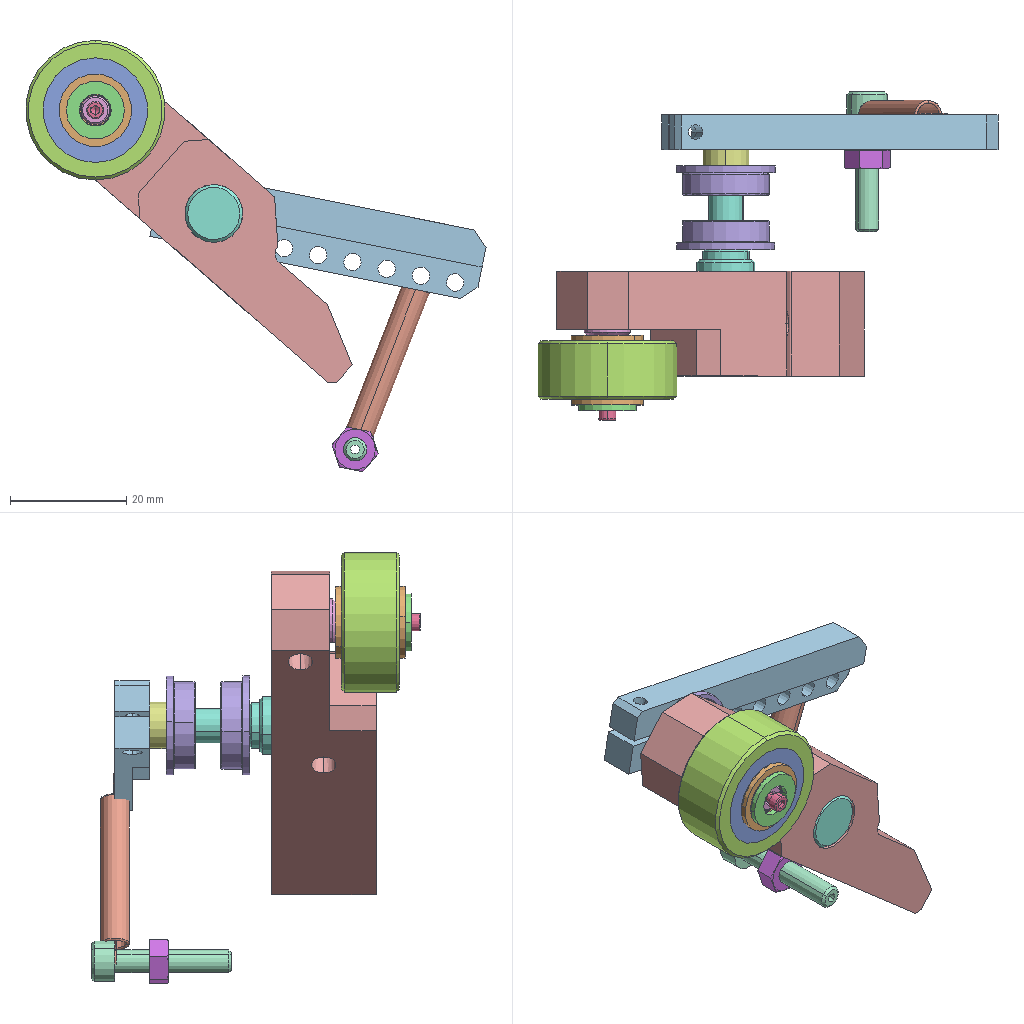Assembly | SolidWorks | 13 different items | 15 placed | box 79 x 56 x 74 mm
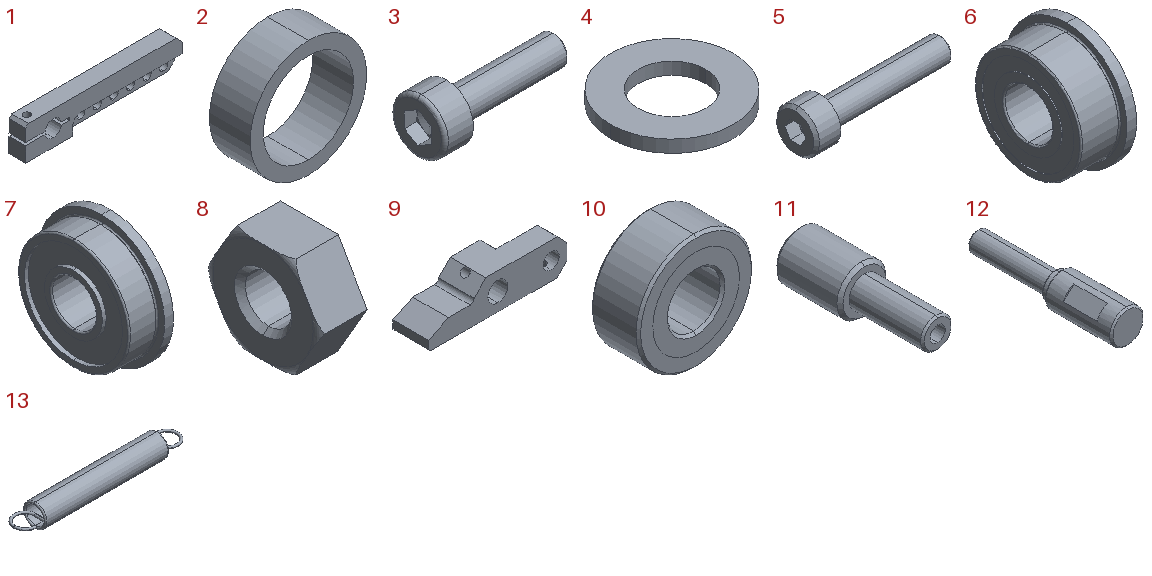Parts list (item | quantity | size | volume | features):
1 | x1 | 57 x 6 x 12 mm | 2922 mm3 | features ICE 4, 3DProfileFeature 2, Chamfer 2, HoleWzd 2, Extrusion 1, Fillet 1, LPattern 1
2 | x1 | 8 x 2.8 x 8 mm | 56.209 mm3 | features Extrusion 1
3 | x1 | 7.6 x 3 x 3 mm | 21.652 mm3 | features Fillet 2, RevCut 2, Boss 1, Chamfer 1, Cut 1, Extrusion 1, LPattern 1
4 | x1 | 10 x 10 x 1 mm | 54.782 mm3 | features Extrusion 1
5 | x1 | 24 x 7 x 7 mm | 346.79 mm3 | features ICE 1, RevCut 1, Revolution 1
6 | x2 | 5 x 12.5 x 12.5 mm | 394.425 mm3 | features RefAxis 3, 3DProfileFeature 1, Revolution 1
7 | x2 | 5 x 17 x 17 mm | 704.07 mm3 | features RefAxis 3, 3DProfileFeature 1, Revolution 1
8 | x1 | 3.2 x 8.083 x 7 mm | 107.662 mm3 | features RefAxis 3, 3DProfileFeature 1, ICE 1, RevCut 1, Revolution 1
9 | x1 | 70 x 18 x 18 mm | 12843 mm3 | features Chamfer 5, ICE 4, HoleWzd 3, 3DProfileFeature 1, CirPattern 1, Extrusion 1, Fillet 1
10 | x1 | 24 x 10 x 24 mm | 3546 mm3 | features Chamfer 3, ICE 2, Extrusion 1
11 | x1 | 8 x 22.8 x 7.5 mm | 720.407 mm3 | features Chamfer 2, Cut 1, Extrusion 1, HoleWzd 1, ICE 1
12 | x1 | 10 x 44.9 x 10 mm | 2272 mm3 | features ICE 5, Chamfer 3, CirPattern 1, Extrusion 1
13 | x1 | 36 x 5 x 5 mm | 195.064 mm3 | features Revolution 5, RefAxis 2
Mates (type | each side: item.copy, entity, surface, feature):
DistanceDim | 10.1 face plane Boss-Extrude1 | 9.1 face plane Boss-Extrude1
Concentric | 10.1 face cylinder Boss-Extrude1 | 9.1 face cylinder Boss-Extrude1
Coincident | 10.1 face plane Boss-Extrude1 | 6.1 face plane Revolve1
Concentric | 10.1 face cylinder Boss-Extrude1 | 6.1 face cylinder Revolve1
Coincident | 10.1 face plane Boss-Extrude1 | 6.2 face plane Revolve1
Concentric | 10.1 face cylinder Boss-Extrude1 | 6.2 face cylinder Revolve1
Coincident | 6.2 face plane Revolve1 | 11.1 face plane Boss-Extrude2
Concentric | 9.1 face cylinder Boss-Extrude1 | 11.1 face cylinder Boss-Extrude2
Concentric | 9.1 face cylinder Cut-Extrude1 | 7.1 face cylinder Revolve1
Concentric | 9.1 face cylinder Cut-Extrude1 | 7.2 face cylinder Revolve1
Concentric | 11.1 face cylinder M3 Tapped Hole1 | 4.1 face cylinder Base-Extrude
Coincident | 11.1 face plane Boss-Extrude1 | 4.1 face plane Base-Extrude
Concentric | 11.1 face cylinder M3 Tapped Hole1 | 3.1 face cylinder BaseBody
Coincident | 4.1 face plane Base-Extrude | 3.1 face plane BaseHead
Concentric | 12.1 face cylinder Boss-Extrude2 | 7.2 face cylinder Revolve1
Coincident | 12.1 face plane Boss-Extrude2 | 7.1 face plane Revolve1
DistanceDim | 7.2 face plane Revolve1 | 7.1 face plane Revolve1
Concentric | 12.1 face cylinder Boss-Extrude3 | 1.1 face cylinder Boss-Extrude1
Coincident | 12.1 face plane Boss-Extrude3 | 1.1 face plane Boss-Extrude1
Coincident | 9.1 face plane Boss-Extrude2 | 12.1 face plane Boss-Extrude1
PlanarAngleDim | 12.1 plane | 1.1 face plane Boss-Extrude1
Concentric | 12.1 face cylinder Boss-Extrude3 | 2.1 face cylinder Boss-Extrude1
Coincident | 7.2 face plane Revolve1 | 2.1 face plane Boss-Extrude1
Coincident | 1.1 face plane Boss-Extrude1 | 5.1 face plane Revolve1
Concentric | 8.1 face cylinder Cut-Revolve1 | 5.1 face cylinder Revolve1
DistanceDim | 8.1 face plane Revolve1 | 5.1 face plane Revolve1
Concentric | 1.1 edge | 13.1 axis
Coincident | 1.1 face plane Boss-Extrude1 | 13.1 plane
PlanarAngleDim | 13.1 plane | 1.1 face plane Cut-Extrude5